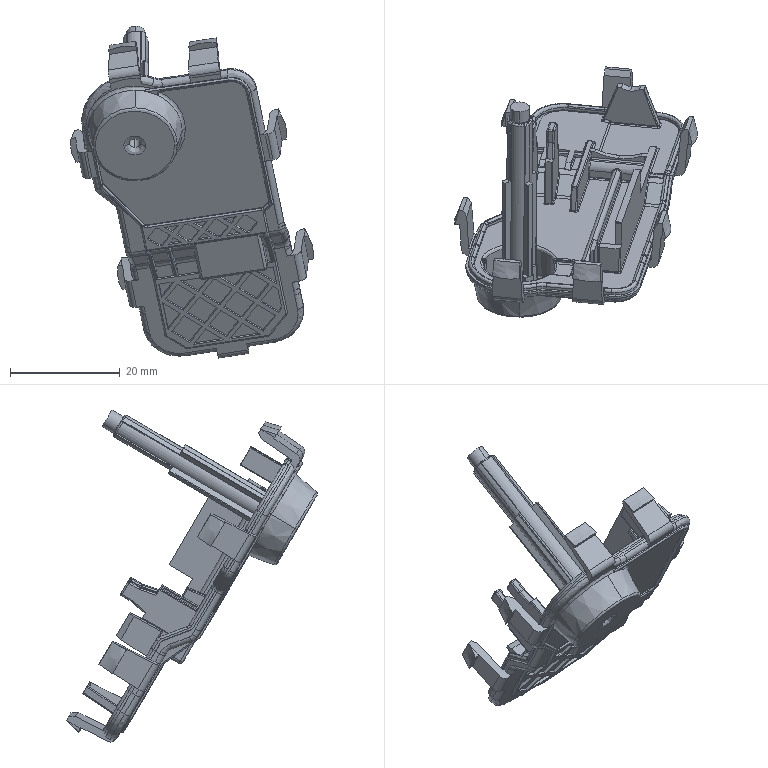Part | STEP file | PN_0002 | 1 solid | 1201 faces | box 44.212 x 45.623 x 60.394 mm | volume 5607 mm3 | cylinder 498 | plane 441 | spline 255 | cone 7 | commonest cylinder face diameters 0.6 x138 0.4 x114 1 x67 2 x44 1.001 x28 0.2 x10